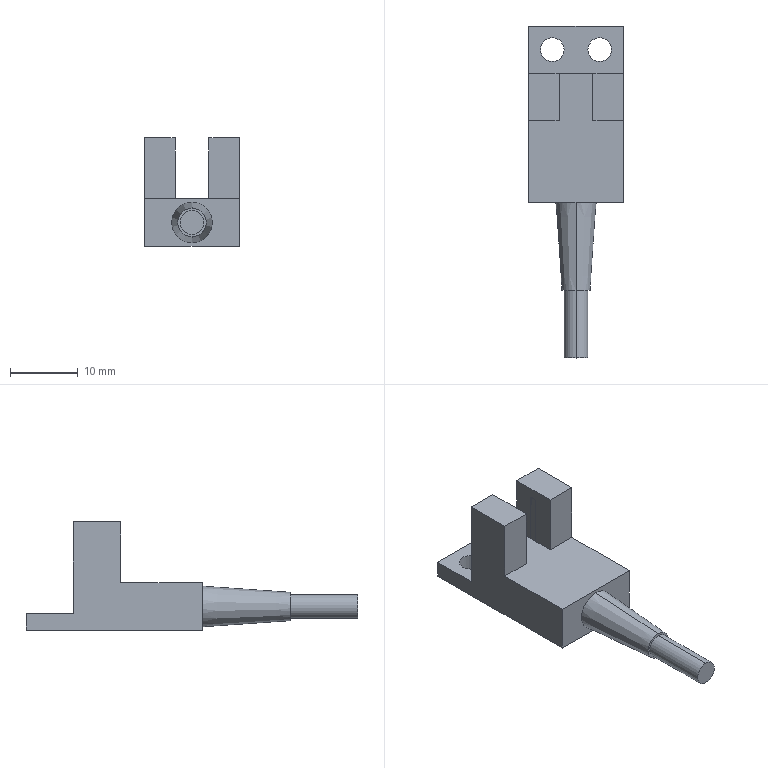Part | NX | features BREP 1 | 1 solid | 32 faces | box 14 x 49 x 16 mm | volume 2990 mm3 | plane 24 | cylinder 6 | cone 2 | commonest cylinder face diameters 3.5 x6
STEP:
#1=CARTESIAN_POINT('',(0.,-38.5,1.75));
#2=VERTEX_POINT('',#1);
#3=CARTESIAN_POINT('',(0.,-38.5,5.25));
#4=VERTEX_POINT('',#3);
#5=CARTESIAN_POINT('',(0.,-38.5,3.5));
#6=DIRECTION('',(0.,1.,0.));
#7=DIRECTION('',(0.,0.,-1.));
#8=AXIS2_PLACEMENT_3D('',#5,#6,#7);
#9=CIRCLE('',#8,1.75);
#10=EDGE_CURVE('',#2,#4,#9,.T.);
#11=ORIENTED_EDGE('',*,*,#10,.F.);
#12=CARTESIAN_POINT('',(0.,-38.5,3.5));
#13=DIRECTION('',(0.,1.,0.));
#14=DIRECTION('',(0.,0.,-1.));
#15=AXIS2_PLACEMENT_3D('',#12,#13,#14);
#16=CIRCLE('',#15,1.75);
#17=EDGE_CURVE('',#4,#2,#16,.T.);
#18=ORIENTED_EDGE('',*,*,#17,.F.);
#19=EDGE_LOOP('',(#11,#18));
#20=FACE_BOUND('',#19,.T.);
#21=CARTESIAN_POINT('',(0.,-38.5,7.));
#22=DIRECTION('',(0.,-1.,0.));
#23=DIRECTION('',(0.,0.,-1.));
#24=AXIS2_PLACEMENT_3D('',#21,#22,#23);
#25=PLANE('',#24);
#26=ADVANCED_FACE('',(#20),#25,.T.);
#27=CARTESIAN_POINT('',(2.45,0.5,7.));
#28=VERTEX_POINT('',#27);
#29=CARTESIAN_POINT('',(2.45,0.5,14.5));
#30=VERTEX_POINT('',#29);
#31=CARTESIAN_POINT('',(2.45,0.5,14.5));
#32=DIRECTION('',(0.,0.,1.));
#33=VECTOR('',#32,1000.);
#34=LINE('',#31,#33);
#35=EDGE_CURVE('',#28,#30,#34,.T.);
#36=ORIENTED_EDGE('',*,*,#35,.F.);
#37=CARTESIAN_POINT('',(2.45,-0.5,7.));
#38=VERTEX_POINT('',#37);
#39=CARTESIAN_POINT('',(2.45,3.5,7.));
#40=DIRECTION('',(0.,-1.,0.));
#41=VECTOR('',#40,1000.);
#42=LINE('',#39,#41);
#43=EDGE_CURVE('',#28,#38,#42,.T.);
#44=ORIENTED_EDGE('',*,*,#43,.T.);
#45=CARTESIAN_POINT('',(2.45,-0.5,14.5));
#46=VERTEX_POINT('',#45);
#47=CARTESIAN_POINT('',(2.45,-0.5,7.));
#48=DIRECTION('',(0.,0.,-1.));
#49=VECTOR('',#48,1000.);
#50=LINE('',#47,#49);
#51=EDGE_CURVE('',#46,#38,#50,.T.);
#52=ORIENTED_EDGE('',*,*,#51,.F.);
#53=CARTESIAN_POINT('',(2.45,-0.5,14.5));
#54=DIRECTION('',(0.,-1.,0.));
#55=VECTOR('',#54,1000.);
#56=LINE('',#53,#55);
#57=EDGE_CURVE('',#30,#46,#56,.T.);
#58=ORIENTED_EDGE('',*,*,#57,.F.);
#59=EDGE_LOOP('',(#36,#44,#52,#58));
#60=FACE_BOUND('',#59,.T.);
#61=CARTESIAN_POINT('',(2.45,3.5,0.));
#62=DIRECTION('',(-1.,0.,0.));
#63=DIRECTION('',(0.,0.,1.));
#64=AXIS2_PLACEMENT_3D('',#61,#62,#63);
#65=PLANE('',#64);
#66=ADVANCED_FACE('',(#60),#65,.T.);
#67=CARTESIAN_POINT('',(-2.45,-0.5,14.5));
#68=VERTEX_POINT('',#67);
#69=CARTESIAN_POINT('',(-2.45,-0.5,7.));
#70=VERTEX_POINT('',#69);
#71=CARTESIAN_POINT('',(-2.45,-0.5,7.));
#72=DIRECTION('',(0.,0.,-1.));
#73=VECTOR('',#72,1000.);
#74=LINE('',#71,#73);
#75=EDGE_CURVE('',#68,#70,#74,.T.);
#76=ORIENTED_EDGE('',*,*,#75,.T.);
#77=CARTESIAN_POINT('',(-2.45,0.5,7.));
#78=VERTEX_POINT('',#77);
#79=CARTESIAN_POINT('',(-2.45,3.5,7.));
#80=DIRECTION('',(0.,-1.,0.));
#81=VECTOR('',#80,1000.);
#82=LINE('',#79,#81);
#83=EDGE_CURVE('',#78,#70,#82,.T.);
#84=ORIENTED_EDGE('',*,*,#83,.F.);
#85=CARTESIAN_POINT('',(-2.45,0.5,14.5));
#86=VERTEX_POINT('',#85);
#87=CARTESIAN_POINT('',(-2.45,0.5,14.5));
#88=DIRECTION('',(0.,0.,1.));
#89=VECTOR('',#88,1000.);
#90=LINE('',#87,#89);
#91=EDGE_CURVE('',#78,#86,#90,.T.);
#92=ORIENTED_EDGE('',*,*,#91,.T.);
#93=CARTESIAN_POINT('',(-2.45,-0.5,14.5));
#94=DIRECTION('',(0.,-1.,0.));
#95=VECTOR('',#94,1000.);
#96=LINE('',#93,#95);
#97=EDGE_CURVE('',#86,#68,#96,.T.);
#98=ORIENTED_EDGE('',*,*,#97,.T.);
#99=EDGE_LOOP('',(#76,#84,#92,#98));
#100=FACE_BOUND('',#99,.T.);
#101=CARTESIAN_POINT('',(-2.45,3.5,0.));
#102=DIRECTION('',(-1.,0.,0.));
#103=DIRECTION('',(0.,0.,1.));
#104=AXIS2_PLACEMENT_3D('',#101,#102,#103);
#105=PLANE('',#104);
#106=ADVANCED_FACE('',(#100),#105,.F.);
#107=CARTESIAN_POINT('',(0.,-28.5,5.25));
#108=VERTEX_POINT('',#107);
#109=CARTESIAN_POINT('',(0.,-28.5,5.25));
#110=DIRECTION('',(0.,-1.,0.));
#111=VECTOR('',#110,1000.);
#112=LINE('',#109,#111);
#113=EDGE_CURVE('',#108,#4,#112,.T.);
#114=ORIENTED_EDGE('',*,*,#113,.F.);
#115=CARTESIAN_POINT('',(0.,-28.5,1.75));
#116=VERTEX_POINT('',#115);
#117=CARTESIAN_POINT('',(0.,-28.5,3.5));
#118=DIRECTION('',(0.,1.,0.));
#119=DIRECTION('',(0.,0.,-1.));
#120=AXIS2_PLACEMENT_3D('',#117,#118,#119);
#121=CIRCLE('',#120,1.75);
#122=EDGE_CURVE('',#116,#108,#121,.T.);
#123=ORIENTED_EDGE('',*,*,#122,.F.);
#124=CARTESIAN_POINT('',(0.,-28.5,1.75));
#125=DIRECTION('',(0.,-1.,0.));
#126=VECTOR('',#125,1000.);
#127=LINE('',#124,#126);
#128=EDGE_CURVE('',#116,#2,#127,.T.);
#129=ORIENTED_EDGE('',*,*,#128,.T.);
#130=ORIENTED_EDGE('',*,*,#10,.T.);
#131=EDGE_LOOP('',(#114,#123,#129,#130));
#132=FACE_BOUND('',#131,.T.);
#133=CARTESIAN_POINT('',(0.,-28.5,3.5));
#134=DIRECTION('',(0.,-1.,0.));
#135=DIRECTION('',(0.,0.,-1.));
#136=AXIS2_PLACEMENT_3D('',#133,#134,#135);
#137=CYLINDRICAL_SURFACE('',#136,1.75);
#138=ADVANCED_FACE('',(#132),#137,.T.);
#139=CARTESIAN_POINT('',(2.5,-0.5,14.5));
#140=VERTEX_POINT('',#139);
#141=CARTESIAN_POINT('',(2.5,-0.5,14.5));
#142=DIRECTION('',(-1.,0.,0.));
#143=VECTOR('',#142,1000.);
#144=LINE('',#141,#143);
#145=EDGE_CURVE('',#140,#46,#144,.T.);
#146=ORIENTED_EDGE('',*,*,#145,.F.);
#147=CARTESIAN_POINT('',(2.5,0.5,14.5));
#148=VERTEX_POINT('',#147);
#149=CARTESIAN_POINT('',(2.5,3.5,14.5));
#150=DIRECTION('',(0.,-1.,0.));
#151=VECTOR('',#150,1000.);
#152=LINE('',#149,#151);
#153=EDGE_CURVE('',#148,#140,#152,.T.);
#154=ORIENTED_EDGE('',*,*,#153,.F.);
#155=CARTESIAN_POINT('',(2.5,0.5,14.5));
#156=DIRECTION('',(1.,0.,0.));
#157=VECTOR('',#156,1000.);
#158=LINE('',#155,#157);
#159=EDGE_CURVE('',#30,#148,#158,.T.);
#160=ORIENTED_EDGE('',*,*,#159,.F.);
#161=ORIENTED_EDGE('',*,*,#57,.T.);
#162=EDGE_LOOP('',(#146,#154,#160,#161));
#163=FACE_BOUND('',#162,.T.);
#164=CARTESIAN_POINT('',(2.5,-0.5,14.5));
#165=DIRECTION('',(0.,0.,1.));
#166=DIRECTION('',(1.,0.,0.));
#167=AXIS2_PLACEMENT_3D('',#164,#165,#166);
#168=PLANE('',#167);
#169=ADVANCED_FACE('',(#163),#168,.T.);
#170=ORIENTED_EDGE('',*,*,#51,.T.);
#171=CARTESIAN_POINT('',(2.5,-0.5,7.));
#172=VERTEX_POINT('',#171);
#173=CARTESIAN_POINT('',(2.5,-0.5,7.));
#174=DIRECTION('',(1.,0.,0.));
#175=VECTOR('',#174,1000.);
#176=LINE('',#173,#175);
#177=EDGE_CURVE('',#38,#172,#176,.T.);
#178=ORIENTED_EDGE('',*,*,#177,.T.);
#179=CARTESIAN_POINT('',(2.5,-0.5,7.));
#180=DIRECTION('',(0.,0.,-1.));
#181=VECTOR('',#180,1000.);
#182=LINE('',#179,#181);
#183=EDGE_CURVE('',#140,#172,#182,.T.);
#184=ORIENTED_EDGE('',*,*,#183,.F.);
#185=ORIENTED_EDGE('',*,*,#145,.T.);
#186=EDGE_LOOP('',(#170,#178,#184,#185));
#187=FACE_BOUND('',#186,.T.);
#188=CARTESIAN_POINT('',(2.5,-0.5,7.));
#189=DIRECTION('',(0.,-1.,0.));
#190=DIRECTION('',(0.,0.,-1.));
#191=AXIS2_PLACEMENT_3D('',#188,#189,#190);
#192=PLANE('',#191);
#193=ADVANCED_FACE('',(#187),#192,.T.);
#194=CARTESIAN_POINT('',(2.5,0.5,7.));
#195=VERTEX_POINT('',#194);
#196=CARTESIAN_POINT('',(2.5,0.5,7.));
#197=DIRECTION('',(0.,0.,1.));
#198=VECTOR('',#197,1000.);
#199=LINE('',#196,#198);
#200=EDGE_CURVE('',#195,#148,#199,.T.);
#201=ORIENTED_EDGE('',*,*,#200,.F.);
#202=CARTESIAN_POINT('',(2.5,0.5,7.));
#203=DIRECTION('',(-1.,0.,0.));
#204=VECTOR('',#203,1000.);
#205=LINE('',#202,#204);
#206=EDGE_CURVE('',#195,#28,#205,.T.);
#207=ORIENTED_EDGE('',*,*,#206,.T.);
#208=ORIENTED_EDGE('',*,*,#35,.T.);
#209=ORIENTED_EDGE('',*,*,#159,.T.);
#210=EDGE_LOOP('',(#201,#207,#208,#209));
#211=FACE_BOUND('',#210,.T.);
#212=CARTESIAN_POINT('',(2.5,0.5,14.5));
#213=DIRECTION('',(0.,1.,0.));
#214=DIRECTION('',(0.,0.,1.));
#215=AXIS2_PLACEMENT_3D('',#212,#213,#214);
#216=PLANE('',#215);
#217=ADVANCED_FACE('',(#211),#216,.T.);
#218=CARTESIAN_POINT('',(-2.5,-0.5,7.));
#219=VERTEX_POINT('',#218);
#220=CARTESIAN_POINT('',(-2.5,-0.5,14.5));
#221=VERTEX_POINT('',#220);
#222=CARTESIAN_POINT('',(-2.5,-0.5,16.));
#223=DIRECTION('',(0.,0.,1.));
#224=VECTOR('',#223,1000.);
#225=LINE('',#222,#224);
#226=EDGE_CURVE('',#219,#221,#225,.T.);
#227=ORIENTED_EDGE('',*,*,#226,.F.);
#228=CARTESIAN_POINT('',(-2.5,-0.5,7.));
#229=DIRECTION('',(-1.,0.,0.));
#230=VECTOR('',#229,1000.);
#231=LINE('',#228,#230);
#232=EDGE_CURVE('',#70,#219,#231,.T.);
#233=ORIENTED_EDGE('',*,*,#232,.F.);
#234=ORIENTED_EDGE('',*,*,#75,.F.);
#235=CARTESIAN_POINT('',(-2.5,-0.5,14.5));
#236=DIRECTION('',(-1.,0.,0.));
#237=VECTOR('',#236,1000.);
#238=LINE('',#235,#237);
#239=EDGE_CURVE('',#68,#221,#238,.T.);
#240=ORIENTED_EDGE('',*,*,#239,.T.);
#241=EDGE_LOOP('',(#227,#233,#234,#240));
#242=FACE_BOUND('',#241,.T.);
#243=CARTESIAN_POINT('',(-2.5,-0.5,7.));
#244=DIRECTION('',(0.,1.,0.));
#245=DIRECTION('',(0.,0.,1.));
#246=AXIS2_PLACEMENT_3D('',#243,#244,#245);
#247=PLANE('',#246);
#248=ADVANCED_FACE('',(#242),#247,.F.);
#249=ORIENTED_EDGE('',*,*,#239,.F.);
#250=ORIENTED_EDGE('',*,*,#97,.F.);
#251=CARTESIAN_POINT('',(-2.5,0.5,14.5));
#252=VERTEX_POINT('',#251);
#253=CARTESIAN_POINT('',(-2.5,0.5,14.5));
#254=DIRECTION('',(-1.,0.,0.));
#255=VECTOR('',#254,1000.);
#256=LINE('',#253,#255);
#257=EDGE_CURVE('',#86,#252,#256,.T.);
#258=ORIENTED_EDGE('',*,*,#257,.T.);
#259=CARTESIAN_POINT('',(-2.5,3.5,14.5));
#260=DIRECTION('',(0.,1.,0.));
#261=VECTOR('',#260,1000.);
#262=LINE('',#259,#261);
#263=EDGE_CURVE('',#221,#252,#262,.T.);
#264=ORIENTED_EDGE('',*,*,#263,.F.);
#265=EDGE_LOOP('',(#249,#250,#258,#264));
#266=FACE_BOUND('',#265,.T.);
#267=CARTESIAN_POINT('',(-2.5,-0.5,14.5));
#268=DIRECTION('',(0.,0.,-1.));
#269=DIRECTION('',(-1.,0.,0.));
#270=AXIS2_PLACEMENT_3D('',#267,#268,#269);
#271=PLANE('',#270);
#272=ADVANCED_FACE('',(#266),#271,.F.);
#273=CARTESIAN_POINT('',(-2.5,0.5,7.));
#274=VERTEX_POINT('',#273);
#275=CARTESIAN_POINT('',(-2.5,0.5,16.));
#276=DIRECTION('',(0.,0.,-1.));
#277=VECTOR('',#276,1000.);
#278=LINE('',#275,#277);
#279=EDGE_CURVE('',#252,#274,#278,.T.);
#280=ORIENTED_EDGE('',*,*,#279,.F.);
#281=ORIENTED_EDGE('',*,*,#257,.F.);
#282=ORIENTED_EDGE('',*,*,#91,.F.);
#283=CARTESIAN_POINT('',(-2.5,0.5,7.));
#284=DIRECTION('',(1.,0.,0.));
#285=VECTOR('',#284,1000.);
#286=LINE('',#283,#285);
#287=EDGE_CURVE('',#274,#78,#286,.T.);
#288=ORIENTED_EDGE('',*,*,#287,.F.);
#289=EDGE_LOOP('',(#280,#281,#282,#288));
#290=FACE_BOUND('',#289,.T.);
#291=CARTESIAN_POINT('',(-2.5,0.5,14.5));
#292=DIRECTION('',(0.,-1.,0.));
#293=DIRECTION('',(0.,0.,-1.));
#294=AXIS2_PLACEMENT_3D('',#291,#292,#293);
#295=PLANE('',#294);
#296=ADVANCED_FACE('',(#290),#295,.F.);
#297=CARTESIAN_POINT('',(0.,-28.5,5.591));
#298=VERTEX_POINT('',#297);
#299=CARTESIAN_POINT('',(0.,-28.5,1.409));
#300=VERTEX_POINT('',#299);
#301=CARTESIAN_POINT('',(0.,-28.5,3.5));
#302=DIRECTION('',(0.,1.,0.));
#303=DIRECTION('',(0.,0.,1.));
#304=AXIS2_PLACEMENT_3D('',#301,#302,#303);
#305=CIRCLE('',#304,2.091);
#306=EDGE_CURVE('',#298,#300,#305,.T.);
#307=ORIENTED_EDGE('',*,*,#306,.F.);
#308=CARTESIAN_POINT('',(0.,-28.5,3.5));
#309=DIRECTION('',(0.,1.,0.));
#310=DIRECTION('',(0.,0.,1.));
#311=AXIS2_PLACEMENT_3D('',#308,#309,#310);
#312=CIRCLE('',#311,2.091);
#313=EDGE_CURVE('',#300,#298,#312,.T.);
#314=ORIENTED_EDGE('',*,*,#313,.F.);
#315=EDGE_LOOP('',(#307,#314));
#316=FACE_BOUND('',#315,.T.);
#317=ORIENTED_EDGE('',*,*,#122,.T.);
#318=CARTESIAN_POINT('',(0.,-28.5,3.5));
#319=DIRECTION('',(0.,1.,0.));
#320=DIRECTION('',(0.,0.,-1.));
#321=AXIS2_PLACEMENT_3D('',#318,#319,#320);
#322=CIRCLE('',#321,1.75);
#323=EDGE_CURVE('',#108,#116,#322,.T.);
#324=ORIENTED_EDGE('',*,*,#323,.T.);
#325=EDGE_LOOP('',(#317,#324));
#326=FACE_BOUND('',#325,.T.);
#327=CARTESIAN_POINT('',(0.,-28.5,7.));
#328=DIRECTION('',(0.,-1.,0.));
#329=DIRECTION('',(0.,0.,-1.));
#330=AXIS2_PLACEMENT_3D('',#327,#328,#329);
#331=PLANE('',#330);
#332=ADVANCED_FACE('',(#316,#326),#331,.T.);
#333=CARTESIAN_POINT('',(2.5,3.5,7.));
#334=VERTEX_POINT('',#333);
#335=CARTESIAN_POINT('',(2.5,3.5,7.));
#336=DIRECTION('',(0.,1.,0.));
#337=VECTOR('',#336,1000.);
#338=LINE('',#335,#337);
#339=EDGE_CURVE('',#195,#334,#338,.T.);
#340=ORIENTED_EDGE('',*,*,#339,.F.);
#341=ORIENTED_EDGE('',*,*,#200,.T.);
#342=ORIENTED_EDGE('',*,*,#153,.T.);
#343=ORIENTED_EDGE('',*,*,#183,.T.);
#344=CARTESIAN_POINT('',(2.5,-3.5,7.));
#345=VERTEX_POINT('',#344);
#346=CARTESIAN_POINT('',(2.5,3.5,7.));
#347=DIRECTION('',(0.,1.,0.));
#348=VECTOR('',#347,1000.);
#349=LINE('',#346,#348);
#350=EDGE_CURVE('',#345,#172,#349,.T.);
#351=ORIENTED_EDGE('',*,*,#350,.F.);
#352=CARTESIAN_POINT('',(2.5,-3.5,16.));
#353=VERTEX_POINT('',#352);
#354=CARTESIAN_POINT('',(2.5,-3.5,0.));
#355=DIRECTION('',(0.,0.,1.));
#356=VECTOR('',#355,1000.);
#357=LINE('',#354,#356);
#358=EDGE_CURVE('',#345,#353,#357,.T.);
#359=ORIENTED_EDGE('',*,*,#358,.T.);
#360=CARTESIAN_POINT('',(2.5,3.5,16.));
#361=VERTEX_POINT('',#360);
#362=CARTESIAN_POINT('',(2.5,3.5,16.));
#363=DIRECTION('',(0.,-1.,0.));
#364=VECTOR('',#363,1000.);
#365=LINE('',#362,#364);
#366=EDGE_CURVE('',#361,#353,#365,.T.);
#367=ORIENTED_EDGE('',*,*,#366,.F.);
#368=CARTESIAN_POINT('',(2.5,3.5,0.));
#369=DIRECTION('',(0.,0.,1.));
#370=VECTOR('',#369,1000.);
#371=LINE('',#368,#370);
#372=EDGE_CURVE('',#334,#361,#371,.T.);
#373=ORIENTED_EDGE('',*,*,#372,.F.);
#374=EDGE_LOOP('',(#340,#341,#342,#343,#351,#359,#367,#373));
#375=FACE_BOUND('',#374,.T.);
#376=CARTESIAN_POINT('',(2.5,3.5,7.));
#377=DIRECTION('',(-1.,0.,0.));
#378=DIRECTION('',(0.,0.,1.));
#379=AXIS2_PLACEMENT_3D('',#376,#377,#378);
#380=PLANE('',#379);
#381=ADVANCED_FACE('',(#375),#380,.T.);
#382=ORIENTED_EDGE('',*,*,#263,.T.);
#383=ORIENTED_EDGE('',*,*,#279,.T.);
#384=CARTESIAN_POINT('',(-2.5,3.5,7.));
#385=VERTEX_POINT('',#384);
#386=CARTESIAN_POINT('',(-2.5,3.5,7.));
#387=DIRECTION('',(0.,-1.,0.));
#388=VECTOR('',#387,1000.);
#389=LINE('',#386,#388);
#390=EDGE_CURVE('',#385,#274,#389,.T.);
#391=ORIENTED_EDGE('',*,*,#390,.F.);
#392=CARTESIAN_POINT('',(-2.5,3.5,16.));
#393=VERTEX_POINT('',#392);
#394=CARTESIAN_POINT('',(-2.5,3.5,0.));
#395=DIRECTION('',(0.,0.,-1.));
#396=VECTOR('',#395,1000.);
#397=LINE('',#394,#396);
#398=EDGE_CURVE('',#393,#385,#397,.T.);
#399=ORIENTED_EDGE('',*,*,#398,.F.);
#400=CARTESIAN_POINT('',(-2.5,-3.5,16.));
#401=VERTEX_POINT('',#400);
#402=CARTESIAN_POINT('',(-2.5,3.5,16.));
#403=DIRECTION('',(0.,1.,0.));
#404=VECTOR('',#403,1000.);
#405=LINE('',#402,#404);
#406=EDGE_CURVE('',#401,#393,#405,.T.);
#407=ORIENTED_EDGE('',*,*,#406,.F.);
#408=CARTESIAN_POINT('',(-2.5,-3.5,7.));
#409=VERTEX_POINT('',#408);
#410=CARTESIAN_POINT('',(-2.5,-3.5,0.));
#411=DIRECTION('',(0.,0.,-1.));
#412=VECTOR('',#411,1000.);
#413=LINE('',#410,#412);
#414=EDGE_CURVE('',#401,#409,#413,.T.);
#415=ORIENTED_EDGE('',*,*,#414,.T.);
#416=CARTESIAN_POINT('',(-2.5,3.5,7.));
#417=DIRECTION('',(0.,-1.,0.));
#418=VECTOR('',#417,1000.);
#419=LINE('',#416,#418);
#420=EDGE_CURVE('',#219,#409,#419,.T.);
#421=ORIENTED_EDGE('',*,*,#420,.F.);
#422=ORIENTED_EDGE('',*,*,#226,.T.);
#423=EDGE_LOOP('',(#382,#383,#391,#399,#407,#415,#421,#422));
#424=FACE_BOUND('',#423,.T.);
#425=CARTESIAN_POINT('',(-2.5,3.5,16.));
#426=DIRECTION('',(1.,0.,0.));
#427=DIRECTION('',(0.,0.,-1.));
#428=AXIS2_PLACEMENT_3D('',#425,#426,#427);
#429=PLANE('',#428);
#430=ADVANCED_FACE('',(#424),#429,.T.);
#431=CARTESIAN_POINT('',(7.,3.5,16.));
#432=VERTEX_POINT('',#431);
#433=CARTESIAN_POINT('',(7.,-3.5,16.));
#434=VERTEX_POINT('',#433);
#435=CARTESIAN_POINT('',(7.,3.5,16.));
#436=DIRECTION('',(0.,-1.,0.));
#437=VECTOR('',#436,1000.);
#438=LINE('',#435,#437);
#439=EDGE_CURVE('',#432,#434,#438,.T.);
#440=ORIENTED_EDGE('',*,*,#439,.F.);
#441=CARTESIAN_POINT('',(0.,3.5,16.));
#442=DIRECTION('',(1.,0.,0.));
#443=VECTOR('',#442,1000.);
#444=LINE('',#441,#443);
#445=EDGE_CURVE('',#361,#432,#444,.T.);
#446=ORIENTED_EDGE('',*,*,#445,.F.);
#447=ORIENTED_EDGE('',*,*,#366,.T.);
#448=CARTESIAN_POINT('',(0.,-3.5,16.));
#449=DIRECTION('',(1.,0.,0.));
#450=VECTOR('',#449,1000.);
#451=LINE('',#448,#450);
#452=EDGE_CURVE('',#353,#434,#451,.T.);
#453=ORIENTED_EDGE('',*,*,#452,.T.);
#454=EDGE_LOOP('',(#440,#446,#447,#453));
#455=FACE_BOUND('',#454,.T.);
#456=CARTESIAN_POINT('',(2.5,3.5,16.));
#457=DIRECTION('',(0.,0.,1.));
#458=DIRECTION('',(1.,0.,0.));
#459=AXIS2_PLACEMENT_3D('',#456,#457,#458);
#460=PLANE('',#459);
#461=ADVANCED_FACE('',(#455),#460,.T.);
#462=ORIENTED_EDGE('',*,*,#452,.F.);
#463=ORIENTED_EDGE('',*,*,#358,.F.);
#464=CARTESIAN_POINT('',(7.,-3.5,7.));
#465=VERTEX_POINT('',#464);
#466=CARTESIAN_POINT('',(-2.5,-3.5,7.));
#467=DIRECTION('',(-1.,0.,0.));
#468=VECTOR('',#467,1000.);
#469=LINE('',#466,#468);
#470=EDGE_CURVE('',#465,#345,#469,.T.);
#471=ORIENTED_EDGE('',*,*,#470,.F.);
#472=CARTESIAN_POINT('',(7.,-3.5,16.));
#473=DIRECTION('',(0.,0.,-1.));
#474=VECTOR('',#473,1000.);
#475=LINE('',#472,#474);
#476=EDGE_CURVE('',#434,#465,#475,.T.);
#477=ORIENTED_EDGE('',*,*,#476,.F.);
#478=EDGE_LOOP('',(#462,#463,#471,#477));
#479=FACE_BOUND('',#478,.T.);
#480=CARTESIAN_POINT('',(0.,-3.5,0.));
#481=DIRECTION('',(0.,1.,0.));
#482=DIRECTION('',(0.,0.,1.));
#483=AXIS2_PLACEMENT_3D('',#480,#481,#482);
#484=PLANE('',#483);
#485=ADVANCED_FACE('',(#479),#484,.F.);
#486=CARTESIAN_POINT('',(0.,-15.5,0.5));
#487=VERTEX_POINT('',#486);
#488=CARTESIAN_POINT('',(0.,-15.5,0.5));
#489=DIRECTION('',(0.,0.9976,-0.06976));
#490=VECTOR('',#489,1000.);
#491=LINE('',#488,#490);
#492=EDGE_CURVE('',#487,#300,#491,.F.);
#493=ORIENTED_EDGE('',*,*,#492,.T.);
#494=ORIENTED_EDGE('',*,*,#313,.T.);
#495=CARTESIAN_POINT('',(0.,-15.5,6.5));
#496=VERTEX_POINT('',#495);
#497=CARTESIAN_POINT('',(0.,-15.5,6.5));
#498=DIRECTION('',(0.,0.9976,0.06976));
#499=VECTOR('',#498,1000.);
#500=LINE('',#497,#499);
#501=EDGE_CURVE('',#496,#298,#500,.F.);
#502=ORIENTED_EDGE('',*,*,#501,.F.);
#503=CARTESIAN_POINT('',(0.,-15.5,3.5));
#504=DIRECTION('',(0.,1.,0.));
#505=DIRECTION('',(0.,0.,1.));
#506=AXIS2_PLACEMENT_3D('',#503,#504,#505);
#507=CIRCLE('',#506,3.);
#508=EDGE_CURVE('',#487,#496,#507,.T.);
#509=ORIENTED_EDGE('',*,*,#508,.F.);
#510=EDGE_LOOP('',(#493,#494,#502,#509));
#511=FACE_BOUND('',#510,.T.);
#512=CARTESIAN_POINT('',(0.,-15.5,3.5));
#513=DIRECTION('',(0.,1.,0.));
#514=DIRECTION('',(0.,0.,1.));
#515=AXIS2_PLACEMENT_3D('',#512,#513,#514);
#516=CONICAL_SURFACE('',#515,3.,0.06981);
#517=ADVANCED_FACE('',(#511),#516,.T.);
#518=CARTESIAN_POINT('',(-7.,-3.5,16.));
#519=VERTEX_POINT('',#518);
#520=CARTESIAN_POINT('',(-7.,-3.5,16.));
#521=DIRECTION('',(1.,0.,0.));
#522=VECTOR('',#521,1000.);
#523=LINE('',#520,#522);
#524=EDGE_CURVE('',#519,#401,#523,.T.);
#525=ORIENTED_EDGE('',*,*,#524,.F.);
#526=CARTESIAN_POINT('',(-7.,-3.5,7.));
#527=VERTEX_POINT('',#526);
#528=CARTESIAN_POINT('',(-7.,-3.5,0.));
#529=DIRECTION('',(0.,0.,1.));
#530=VECTOR('',#529,1000.);
#531=LINE('',#528,#530);
#532=EDGE_CURVE('',#527,#519,#531,.T.);
#533=ORIENTED_EDGE('',*,*,#532,.F.);
#534=CARTESIAN_POINT('',(-2.5,-3.5,7.));
#535=DIRECTION('',(-1.,0.,0.));
#536=VECTOR('',#535,1000.);
#537=LINE('',#534,#536);
#538=EDGE_CURVE('',#409,#527,#537,.T.);
#539=ORIENTED_EDGE('',*,*,#538,.F.);
#540=ORIENTED_EDGE('',*,*,#414,.F.);
#541=EDGE_LOOP('',(#525,#533,#539,#540));
#542=FACE_BOUND('',#541,.T.);
#543=CARTESIAN_POINT('',(0.,-3.5,0.));
#544=DIRECTION('',(0.,1.,0.));
#545=DIRECTION('',(0.,0.,1.));
#546=AXIS2_PLACEMENT_3D('',#543,#544,#545);
#547=PLANE('',#546);
#548=ADVANCED_FACE('',(#542),#547,.F.);
#549=ORIENTED_EDGE('',*,*,#406,.T.);
#550=CARTESIAN_POINT('',(-7.,3.5,16.));
#551=VERTEX_POINT('',#550);
#552=CARTESIAN_POINT('',(0.,3.5,16.));
#553=DIRECTION('',(1.,0.,0.));
#554=VECTOR('',#553,1000.);
#555=LINE('',#552,#554);
#556=EDGE_CURVE('',#551,#393,#555,.T.);
#557=ORIENTED_EDGE('',*,*,#556,.F.);
#558=CARTESIAN_POINT('',(-7.,3.5,16.));
#559=DIRECTION('',(0.,1.,0.));
#560=VECTOR('',#559,1000.);
#561=LINE('',#558,#560);
#562=EDGE_CURVE('',#519,#551,#561,.T.);
#563=ORIENTED_EDGE('',*,*,#562,.F.);
#564=ORIENTED_EDGE('',*,*,#524,.T.);
#565=EDGE_LOOP('',(#549,#557,#563,#564));
#566=FACE_BOUND('',#565,.T.);
#567=CARTESIAN_POINT('',(-7.,3.5,16.));
#568=DIRECTION('',(0.,0.,1.));
#569=DIRECTION('',(1.,0.,0.));
#570=AXIS2_PLACEMENT_3D('',#567,#568,#569);
#571=PLANE('',#570);
#572=ADVANCED_FACE('',(#566),#571,.T.);
#573=CARTESIAN_POINT('',(7.,3.5,2.5));
#574=VERTEX_POINT('',#573);
#575=CARTESIAN_POINT('',(7.,3.5,16.));
#576=DIRECTION('',(0.,0.,1.));
#577=VECTOR('',#576,1000.);
#578=LINE('',#575,#577);
#579=EDGE_CURVE('',#574,#432,#578,.T.);
#580=ORIENTED_EDGE('',*,*,#579,.F.);
#581=CARTESIAN_POINT('',(-7.,3.5,2.5));
#582=VERTEX_POINT('',#581);
#583=CARTESIAN_POINT('',(0.,3.5,2.5));
#584=DIRECTION('',(-1.,0.,0.));
#585=VECTOR('',#584,1000.);
#586=LINE('',#583,#585);
#587=EDGE_CURVE('',#574,#582,#586,.T.);
#588=ORIENTED_EDGE('',*,*,#587,.T.);
#589=CARTESIAN_POINT('',(-7.,3.5,0.));
#590=DIRECTION('',(0.,0.,-1.));
#591=VECTOR('',#590,1000.);
#592=LINE('',#589,#591);
#593=EDGE_CURVE('',#551,#582,#592,.T.);
#594=ORIENTED_EDGE('',*,*,#593,.F.);
#595=ORIENTED_EDGE('',*,*,#556,.T.);
#596=ORIENTED_EDGE('',*,*,#398,.T.);
#597=CARTESIAN_POINT('',(-2.5,3.5,7.));
#598=DIRECTION('',(-1.,0.,0.));
#599=VECTOR('',#598,1000.);
#600=LINE('',#597,#599);
#601=EDGE_CURVE('',#334,#385,#600,.T.);
#602=ORIENTED_EDGE('',*,*,#601,.F.);
#603=ORIENTED_EDGE('',*,*,#372,.T.);
#604=ORIENTED_EDGE('',*,*,#445,.T.);
#605=EDGE_LOOP('',(#580,#588,#594,#595,#596,#602,#603,#604));
#606=FACE_BOUND('',#605,.T.);
#607=CARTESIAN_POINT('',(0.,3.5,0.));
#608=DIRECTION('',(0.,1.,0.));
#609=DIRECTION('',(0.,0.,1.));
#610=AXIS2_PLACEMENT_3D('',#607,#608,#609);
#611=PLANE('',#610);
#612=ADVANCED_FACE('',(#606),#611,.T.);
#613=CARTESIAN_POINT('',(7.,-15.5,7.));
#614=VERTEX_POINT('',#613);
#615=CARTESIAN_POINT('',(-7.,-15.5,7.));
#616=VERTEX_POINT('',#615);
#617=CARTESIAN_POINT('',(0.,-15.5,7.));
#618=DIRECTION('',(-1.,0.,0.));
#619=VECTOR('',#618,1000.);
#620=LINE('',#617,#619);
#621=EDGE_CURVE('',#614,#616,#620,.T.);
#622=ORIENTED_EDGE('',*,*,#621,.F.);
#623=CARTESIAN_POINT('',(7.,3.5,7.));
#624=DIRECTION('',(0.,-1.,0.));
#625=VECTOR('',#624,1000.);
#626=LINE('',#623,#625);
#627=EDGE_CURVE('',#465,#614,#626,.T.);
#628=ORIENTED_EDGE('',*,*,#627,.F.);
#629=ORIENTED_EDGE('',*,*,#470,.T.);
#630=ORIENTED_EDGE('',*,*,#350,.T.);
#631=ORIENTED_EDGE('',*,*,#177,.F.);
#632=ORIENTED_EDGE('',*,*,#43,.F.);
#633=ORIENTED_EDGE('',*,*,#206,.F.);
#634=ORIENTED_EDGE('',*,*,#339,.T.);
#635=ORIENTED_EDGE('',*,*,#601,.T.);
#636=ORIENTED_EDGE('',*,*,#390,.T.);
#637=ORIENTED_EDGE('',*,*,#287,.T.);
#638=ORIENTED_EDGE('',*,*,#83,.T.);
#639=ORIENTED_EDGE('',*,*,#232,.T.);
#640=ORIENTED_EDGE('',*,*,#420,.T.);
#641=ORIENTED_EDGE('',*,*,#538,.T.);
#642=CARTESIAN_POINT('',(-7.,3.5,7.));
#643=DIRECTION('',(0.,1.,0.));
#644=VECTOR('',#643,1000.);
#645=LINE('',#642,#644);
#646=EDGE_CURVE('',#616,#527,#645,.T.);
#647=ORIENTED_EDGE('',*,*,#646,.F.);
#648=EDGE_LOOP('',(#622,#628,#629,#630,#631,#632,#633,#634,#635,#636,#637,#638,#639,#640,#641,#647));
#649=FACE_BOUND('',#648,.T.);
#650=CARTESIAN_POINT('',(-2.5,3.5,7.));
#651=DIRECTION('',(0.,0.,1.));
#652=DIRECTION('',(1.,0.,0.));
#653=AXIS2_PLACEMENT_3D('',#650,#651,#652);
#654=PLANE('',#653);
#655=ADVANCED_FACE('',(#649),#654,.T.);
#656=CARTESIAN_POINT('',(-7.,10.5,2.5));
#657=VERTEX_POINT('',#656);
#658=CARTESIAN_POINT('',(7.,10.5,2.5));
#659=VERTEX_POINT('',#658);
#660=CARTESIAN_POINT('',(-7.,10.5,2.5));
#661=DIRECTION('',(1.,0.,0.));
#662=VECTOR('',#661,1000.);
#663=LINE('',#660,#662);
#664=EDGE_CURVE('',#657,#659,#663,.T.);
#665=ORIENTED_EDGE('',*,*,#664,.F.);
#666=CARTESIAN_POINT('',(-7.,3.5,2.5));
#667=DIRECTION('',(0.,1.,0.));
#668=VECTOR('',#667,1000.);
#669=LINE('',#666,#668);
#670=EDGE_CURVE('',#582,#657,#669,.T.);
#671=ORIENTED_EDGE('',*,*,#670,.F.);
#672=ORIENTED_EDGE('',*,*,#587,.F.);
#673=CARTESIAN_POINT('',(7.,3.5,2.5));
#674=DIRECTION('',(0.,-1.,0.));
#675=VECTOR('',#674,1000.);
#676=LINE('',#673,#675);
#677=EDGE_CURVE('',#659,#574,#676,.T.);
#678=ORIENTED_EDGE('',*,*,#677,.F.);
#679=EDGE_LOOP('',(#665,#671,#672,#678));
#680=FACE_BOUND('',#679,.T.);
#681=CARTESIAN_POINT('',(5.25,7.,2.5));
#682=VERTEX_POINT('',#681);
#683=CARTESIAN_POINT('',(1.75,7.,2.5));
#684=VERTEX_POINT('',#683);
#685=CARTESIAN_POINT('',(3.5,7.,2.5));
#686=DIRECTION('',(0.,0.,-1.));
#687=DIRECTION('',(1.,0.,0.));
#688=AXIS2_PLACEMENT_3D('',#685,#686,#687);
#689=CIRCLE('',#688,1.75);
#690=EDGE_CURVE('',#682,#684,#689,.T.);
#691=ORIENTED_EDGE('',*,*,#690,.T.);
#692=CARTESIAN_POINT('',(3.5,7.,2.5));
#693=DIRECTION('',(0.,0.,-1.));
#694=DIRECTION('',(1.,0.,0.));
#695=AXIS2_PLACEMENT_3D('',#692,#693,#694);
#696=CIRCLE('',#695,1.75);
#697=EDGE_CURVE('',#684,#682,#696,.T.);
#698=ORIENTED_EDGE('',*,*,#697,.T.);
#699=EDGE_LOOP('',(#691,#698));
#700=FACE_BOUND('',#699,.T.);
#701=CARTESIAN_POINT('',(-1.75,7.,2.5));
#702=VERTEX_POINT('',#701);
#703=CARTESIAN_POINT('',(-5.25,7.,2.5));
#704=VERTEX_POINT('',#703);
#705=CARTESIAN_POINT('',(-3.5,7.,2.5));
#706=DIRECTION('',(0.,0.,-1.));
#707=DIRECTION('',(1.,0.,0.));
#708=AXIS2_PLACEMENT_3D('',#705,#706,#707);
#709=CIRCLE('',#708,1.75);
#710=EDGE_CURVE('',#702,#704,#709,.T.);
#711=ORIENTED_EDGE('',*,*,#710,.T.);
#712=CARTESIAN_POINT('',(-3.5,7.,2.5));
#713=DIRECTION('',(0.,0.,-1.));
#714=DIRECTION('',(1.,0.,0.));
#715=AXIS2_PLACEMENT_3D('',#712,#713,#714);
#716=CIRCLE('',#715,1.75);
#717=EDGE_CURVE('',#704,#702,#716,.T.);
#718=ORIENTED_EDGE('',*,*,#717,.T.);
#719=EDGE_LOOP('',(#711,#718));
#720=FACE_BOUND('',#719,.T.);
#721=CARTESIAN_POINT('',(0.,3.5,2.5));
#722=DIRECTION('',(0.,0.,-1.));
#723=DIRECTION('',(-1.,0.,0.));
#724=AXIS2_PLACEMENT_3D('',#721,#722,#723);
#725=PLANE('',#724);
#726=ADVANCED_FACE('',(#680,#700,#720),#725,.F.);
#727=CARTESIAN_POINT('',(7.,10.5,0.));
#728=VERTEX_POINT('',#727);
#729=CARTESIAN_POINT('',(7.,10.5,16.));
#730=DIRECTION('',(0.,0.,1.));
#731=VECTOR('',#730,1000.);
#732=LINE('',#729,#731);
#733=EDGE_CURVE('',#728,#659,#732,.T.);
#734=ORIENTED_EDGE('',*,*,#733,.F.);
#735=CARTESIAN_POINT('',(-7.,10.5,0.));
#736=VERTEX_POINT('',#735);
#737=CARTESIAN_POINT('',(7.,10.5,0.));
#738=DIRECTION('',(1.,0.,0.));
#739=VECTOR('',#738,1000.);
#740=LINE('',#737,#739);
#741=EDGE_CURVE('',#736,#728,#740,.T.);
#742=ORIENTED_EDGE('',*,*,#741,.F.);
#743=CARTESIAN_POINT('',(-7.,10.5,0.));
#744=DIRECTION('',(0.,0.,-1.));
#745=VECTOR('',#744,1000.);
#746=LINE('',#743,#745);
#747=EDGE_CURVE('',#657,#736,#746,.T.);
#748=ORIENTED_EDGE('',*,*,#747,.F.);
#749=ORIENTED_EDGE('',*,*,#664,.T.);
#750=EDGE_LOOP('',(#734,#742,#748,#749));
#751=FACE_BOUND('',#750,.T.);
#752=CARTESIAN_POINT('',(-7.,10.5,0.));
#753=DIRECTION('',(0.,1.,0.));
#754=DIRECTION('',(0.,0.,1.));
#755=AXIS2_PLACEMENT_3D('',#752,#753,#754);
#756=PLANE('',#755);
#757=ADVANCED_FACE('',(#751),#756,.T.);
#758=CARTESIAN_POINT('',(7.,-15.5,0.));
#759=VERTEX_POINT('',#758);
#760=CARTESIAN_POINT('',(7.,-15.5,7.));
#761=DIRECTION('',(0.,0.,1.));
#762=VECTOR('',#761,1000.);
#763=LINE('',#760,#762);
#764=EDGE_CURVE('',#759,#614,#763,.T.);
#765=ORIENTED_EDGE('',*,*,#764,.F.);
#766=CARTESIAN_POINT('',(7.,3.5,0.));
#767=DIRECTION('',(0.,-1.,0.));
#768=VECTOR('',#767,1000.);
#769=LINE('',#766,#768);
#770=EDGE_CURVE('',#728,#759,#769,.T.);
#771=ORIENTED_EDGE('',*,*,#770,.F.);
#772=ORIENTED_EDGE('',*,*,#733,.T.);
#773=ORIENTED_EDGE('',*,*,#677,.T.);
#774=ORIENTED_EDGE('',*,*,#579,.T.);
#775=ORIENTED_EDGE('',*,*,#439,.T.);
#776=ORIENTED_EDGE('',*,*,#476,.T.);
#777=ORIENTED_EDGE('',*,*,#627,.T.);
#778=EDGE_LOOP('',(#765,#771,#772,#773,#774,#775,#776,#777));
#779=FACE_BOUND('',#778,.T.);
#780=CARTESIAN_POINT('',(7.,3.5,16.));
#781=DIRECTION('',(1.,0.,0.));
#782=DIRECTION('',(0.,0.,-1.));
#783=AXIS2_PLACEMENT_3D('',#780,#781,#782);
#784=PLANE('',#783);
#785=ADVANCED_FACE('',(#779),#784,.T.);
#786=ORIENTED_EDGE('',*,*,#621,.T.);
#787=CARTESIAN_POINT('',(-7.,-15.5,0.));
#788=VERTEX_POINT('',#787);
#789=CARTESIAN_POINT('',(-7.,-15.5,0.));
#790=DIRECTION('',(0.,0.,1.));
#791=VECTOR('',#790,1000.);
#792=LINE('',#789,#791);
#793=EDGE_CURVE('',#788,#616,#792,.T.);
#794=ORIENTED_EDGE('',*,*,#793,.F.);
#795=CARTESIAN_POINT('',(7.,-15.5,0.));
#796=DIRECTION('',(-1.,0.,0.));
#797=VECTOR('',#796,1000.);
#798=LINE('',#795,#797);
#799=EDGE_CURVE('',#759,#788,#798,.T.);
#800=ORIENTED_EDGE('',*,*,#799,.F.);
#801=ORIENTED_EDGE('',*,*,#764,.T.);
#802=EDGE_LOOP('',(#786,#794,#800,#801));
#803=FACE_BOUND('',#802,.T.);
#804=CARTESIAN_POINT('',(0.,-15.5,3.5));
#805=DIRECTION('',(0.,1.,0.));
#806=DIRECTION('',(0.,0.,1.));
#807=AXIS2_PLACEMENT_3D('',#804,#805,#806);
#808=CIRCLE('',#807,3.);
#809=EDGE_CURVE('',#496,#487,#808,.T.);
#810=ORIENTED_EDGE('',*,*,#809,.T.);
#811=ORIENTED_EDGE('',*,*,#508,.T.);
#812=EDGE_LOOP('',(#810,#811));
#813=FACE_BOUND('',#812,.T.);
#814=CARTESIAN_POINT('',(0.,-15.5,7.));
#815=DIRECTION('',(0.,-1.,0.));
#816=DIRECTION('',(0.,0.,-1.));
#817=AXIS2_PLACEMENT_3D('',#814,#815,#816);
#818=PLANE('',#817);
#819=ADVANCED_FACE('',(#803,#813),#818,.T.);
#820=ORIENTED_EDGE('',*,*,#793,.T.);
#821=ORIENTED_EDGE('',*,*,#646,.T.);
#822=ORIENTED_EDGE('',*,*,#532,.T.);
#823=ORIENTED_EDGE('',*,*,#562,.T.);
#824=ORIENTED_EDGE('',*,*,#593,.T.);
#825=ORIENTED_EDGE('',*,*,#670,.T.);
#826=ORIENTED_EDGE('',*,*,#747,.T.);
#827=CARTESIAN_POINT('',(-7.,3.5,0.));
#828=DIRECTION('',(0.,1.,0.));
#829=VECTOR('',#828,1000.);
#830=LINE('',#827,#829);
#831=EDGE_CURVE('',#788,#736,#830,.T.);
#832=ORIENTED_EDGE('',*,*,#831,.F.);
#833=EDGE_LOOP('',(#820,#821,#822,#823,#824,#825,#826,#832));
#834=FACE_BOUND('',#833,.T.);
#835=CARTESIAN_POINT('',(-7.,3.5,0.));
#836=DIRECTION('',(-1.,0.,0.));
#837=DIRECTION('',(0.,0.,1.));
#838=AXIS2_PLACEMENT_3D('',#835,#836,#837);
#839=PLANE('',#838);
#840=ADVANCED_FACE('',(#834),#839,.T.);
#841=CARTESIAN_POINT('',(-5.25,7.,0.));
#842=VERTEX_POINT('',#841);
#843=CARTESIAN_POINT('',(-5.25,7.,2.5));
#844=DIRECTION('',(0.,0.,1.));
#845=VECTOR('',#844,1000.);
#846=LINE('',#843,#845);
#847=EDGE_CURVE('',#704,#842,#846,.F.);
#848=ORIENTED_EDGE('',*,*,#847,.T.);
#849=CARTESIAN_POINT('',(-1.75,7.,0.));
#850=VERTEX_POINT('',#849);
#851=CARTESIAN_POINT('',(-3.5,7.,0.));
#852=DIRECTION('',(0.,0.,1.));
#853=DIRECTION('',(1.,0.,0.));
#854=AXIS2_PLACEMENT_3D('',#851,#852,#853);
#855=CIRCLE('',#854,1.75);
#856=EDGE_CURVE('',#850,#842,#855,.T.);
#857=ORIENTED_EDGE('',*,*,#856,.F.);
#858=CARTESIAN_POINT('',(-1.75,7.,2.5));
#859=DIRECTION('',(0.,0.,1.));
#860=VECTOR('',#859,1000.);
#861=LINE('',#858,#860);
#862=EDGE_CURVE('',#702,#850,#861,.F.);
#863=ORIENTED_EDGE('',*,*,#862,.F.);
#864=ORIENTED_EDGE('',*,*,#717,.F.);
#865=EDGE_LOOP('',(#848,#857,#863,#864));
#866=FACE_BOUND('',#865,.T.);
#867=CARTESIAN_POINT('',(-3.5,7.,2.5));
#868=DIRECTION('',(0.,0.,1.));
#869=DIRECTION('',(1.,0.,0.));
#870=AXIS2_PLACEMENT_3D('',#867,#868,#869);
#871=CYLINDRICAL_SURFACE('',#870,1.75);
#872=ADVANCED_FACE('',(#866),#871,.F.);
#873=CARTESIAN_POINT('',(1.75,7.,0.));
#874=VERTEX_POINT('',#873);
#875=CARTESIAN_POINT('',(1.75,7.,2.5));
#876=DIRECTION('',(0.,0.,1.));
#877=VECTOR('',#876,1000.);
#878=LINE('',#875,#877);
#879=EDGE_CURVE('',#684,#874,#878,.F.);
#880=ORIENTED_EDGE('',*,*,#879,.T.);
#881=CARTESIAN_POINT('',(5.25,7.,0.));
#882=VERTEX_POINT('',#881);
#883=CARTESIAN_POINT('',(3.5,7.,0.));
#884=DIRECTION('',(0.,0.,1.));
#885=DIRECTION('',(1.,0.,0.));
#886=AXIS2_PLACEMENT_3D('',#883,#884,#885);
#887=CIRCLE('',#886,1.75);
#888=EDGE_CURVE('',#882,#874,#887,.T.);
#889=ORIENTED_EDGE('',*,*,#888,.F.);
#890=CARTESIAN_POINT('',(5.25,7.,2.5));
#891=DIRECTION('',(0.,0.,1.));
#892=VECTOR('',#891,1000.);
#893=LINE('',#890,#892);
#894=EDGE_CURVE('',#682,#882,#893,.F.);
#895=ORIENTED_EDGE('',*,*,#894,.F.);
#896=ORIENTED_EDGE('',*,*,#697,.F.);
#897=EDGE_LOOP('',(#880,#889,#895,#896));
#898=FACE_BOUND('',#897,.T.);
#899=CARTESIAN_POINT('',(3.5,7.,2.5));
#900=DIRECTION('',(0.,0.,1.));
#901=DIRECTION('',(1.,0.,0.));
#902=AXIS2_PLACEMENT_3D('',#899,#900,#901);
#903=CYLINDRICAL_SURFACE('',#902,1.75);
#904=ADVANCED_FACE('',(#898),#903,.F.);
#905=ORIENTED_EDGE('',*,*,#799,.T.);
#906=ORIENTED_EDGE('',*,*,#831,.T.);
#907=ORIENTED_EDGE('',*,*,#741,.T.);
#908=ORIENTED_EDGE('',*,*,#770,.T.);
#909=EDGE_LOOP('',(#905,#906,#907,#908));
#910=FACE_BOUND('',#909,.T.);
#911=ORIENTED_EDGE('',*,*,#856,.T.);
#912=CARTESIAN_POINT('',(-3.5,7.,0.));
#913=DIRECTION('',(0.,0.,1.));
#914=DIRECTION('',(1.,0.,0.));
#915=AXIS2_PLACEMENT_3D('',#912,#913,#914);
#916=CIRCLE('',#915,1.75);
#917=EDGE_CURVE('',#842,#850,#916,.T.);
#918=ORIENTED_EDGE('',*,*,#917,.T.);
#919=EDGE_LOOP('',(#911,#918));
#920=FACE_BOUND('',#919,.T.);
#921=ORIENTED_EDGE('',*,*,#888,.T.);
#922=CARTESIAN_POINT('',(3.5,7.,0.));
#923=DIRECTION('',(0.,0.,1.));
#924=DIRECTION('',(1.,0.,0.));
#925=AXIS2_PLACEMENT_3D('',#922,#923,#924);
#926=CIRCLE('',#925,1.75);
#927=EDGE_CURVE('',#874,#882,#926,.T.);
#928=ORIENTED_EDGE('',*,*,#927,.T.);
#929=EDGE_LOOP('',(#921,#928));
#930=FACE_BOUND('',#929,.T.);
#931=CARTESIAN_POINT('',(7.,3.5,0.));
#932=DIRECTION('',(0.,0.,-1.));
#933=DIRECTION('',(-1.,0.,0.));
#934=AXIS2_PLACEMENT_3D('',#931,#932,#933);
#935=PLANE('',#934);
#936=ADVANCED_FACE('',(#910,#920,#930),#935,.T.);
#937=ORIENTED_EDGE('',*,*,#323,.F.);
#938=ORIENTED_EDGE('',*,*,#113,.T.);
#939=ORIENTED_EDGE('',*,*,#17,.T.);
#940=ORIENTED_EDGE('',*,*,#128,.F.);
#941=EDGE_LOOP('',(#937,#938,#939,#940));
#942=FACE_BOUND('',#941,.T.);
#943=CARTESIAN_POINT('',(0.,-28.5,3.5));
#944=DIRECTION('',(0.,-1.,0.));
#945=DIRECTION('',(0.,0.,-1.));
#946=AXIS2_PLACEMENT_3D('',#943,#944,#945);
#947=CYLINDRICAL_SURFACE('',#946,1.75);
#948=ADVANCED_FACE('',(#942),#947,.T.);
#949=ORIENTED_EDGE('',*,*,#306,.T.);
#950=ORIENTED_EDGE('',*,*,#492,.F.);
#951=ORIENTED_EDGE('',*,*,#809,.F.);
#952=ORIENTED_EDGE('',*,*,#501,.T.);
#953=EDGE_LOOP('',(#949,#950,#951,#952));
#954=FACE_BOUND('',#953,.T.);
#955=CARTESIAN_POINT('',(0.,-15.5,3.5));
#956=DIRECTION('',(0.,1.,0.));
#957=DIRECTION('',(0.,0.,1.));
#958=AXIS2_PLACEMENT_3D('',#955,#956,#957);
#959=CONICAL_SURFACE('',#958,3.,0.06981);
#960=ADVANCED_FACE('',(#954),#959,.T.);
#961=ORIENTED_EDGE('',*,*,#917,.F.);
#962=ORIENTED_EDGE('',*,*,#847,.F.);
#963=ORIENTED_EDGE('',*,*,#710,.F.);
#964=ORIENTED_EDGE('',*,*,#862,.T.);
#965=EDGE_LOOP('',(#961,#962,#963,#964));
#966=FACE_BOUND('',#965,.T.);
#967=CARTESIAN_POINT('',(-3.5,7.,2.5));
#968=DIRECTION('',(0.,0.,1.));
#969=DIRECTION('',(1.,0.,0.));
#970=AXIS2_PLACEMENT_3D('',#967,#968,#969);
#971=CYLINDRICAL_SURFACE('',#970,1.75);
#972=ADVANCED_FACE('',(#966),#971,.F.);
#973=ORIENTED_EDGE('',*,*,#927,.F.);
#974=ORIENTED_EDGE('',*,*,#879,.F.);
#975=ORIENTED_EDGE('',*,*,#690,.F.);
#976=ORIENTED_EDGE('',*,*,#894,.T.);
#977=EDGE_LOOP('',(#973,#974,#975,#976));
#978=FACE_BOUND('',#977,.T.);
#979=CARTESIAN_POINT('',(3.5,7.,2.5));
#980=DIRECTION('',(0.,0.,1.));
#981=DIRECTION('',(1.,0.,0.));
#982=AXIS2_PLACEMENT_3D('',#979,#980,#981);
#983=CYLINDRICAL_SURFACE('',#982,1.75);
#984=ADVANCED_FACE('',(#978),#983,.F.);
#985=CLOSED_SHELL('',(#26,#66,#106,#138,#169,#193,#217,#248,#272,#296,#332,#381,#430,#461,#485,#517,#548,#572,#612,#655,#726,#757,#785,#819,#840,#872,#904,#936,#948,#960,#972,#984));
#986=MANIFOLD_SOLID_BREP('',#985);
#987=(LENGTH_UNIT()NAMED_UNIT(*)SI_UNIT(.MILLI.,.METRE.));
#988=UNCERTAINTY_MEASURE_WITH_UNIT(LENGTH_MEASURE(0.00001),#987,'','');
#989=(NAMED_UNIT(*)PLANE_ANGLE_UNIT()SI_UNIT($,.RADIAN.));
#990=(NAMED_UNIT(*)SI_UNIT($,.STERADIAN.)SOLID_ANGLE_UNIT());
#991=(GEOMETRIC_REPRESENTATION_CONTEXT(3)GLOBAL_UNCERTAINTY_ASSIGNED_CONTEXT((#988))GLOBAL_UNIT_ASSIGNED_CONTEXT((#987,#989,#990))REPRESENTATION_CONTEXT('',''));
#992=ADVANCED_BREP_SHAPE_REPRESENTATION('',(#986),#991);